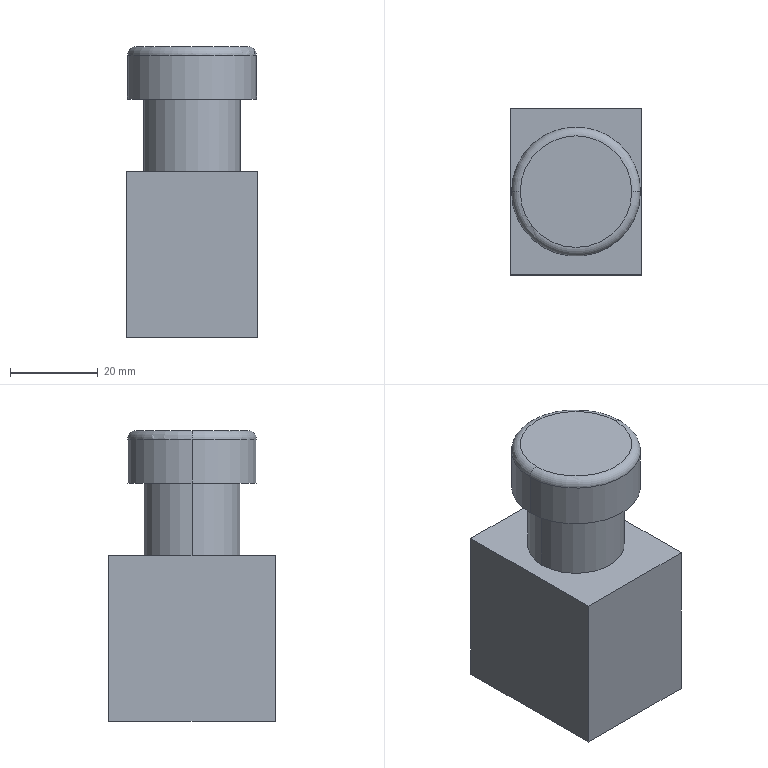Part | STEP file | illuminated flat push button white 24V | 1 solid | 14 faces | box 30 x 38 x 66.5 mm | volume 57717 mm3 | plane 8 | cylinder 4 | torus 2 | commonest cylinder face diameters 22 x2 29.5 x2
STEP:
#1=CARTESIAN_POINT('',(0.,0.,0.));
#2=DIRECTION('',(0.,0.,1.));
#3=DIRECTION('',(1.,0.,0.));
#4=AXIS2_PLACEMENT_3D('',#1,#2,#3);
#5=CARTESIAN_POINT('',(-14.75,0.,10.));
#6=VERTEX_POINT('',#5);
#7=CARTESIAN_POINT('',(14.75,0.,10.));
#8=VERTEX_POINT('',#7);
#9=CARTESIAN_POINT('',(0.,0.,10.));
#10=DIRECTION('',(0.,0.,-1.));
#11=DIRECTION('',(1.,0.,0.));
#12=AXIS2_PLACEMENT_3D('',#9,#10,#11);
#13=CIRCLE('',#12,14.75);
#14=CARTESIAN_POINT('',(0.,0.,10.));
#15=DIRECTION('',(0.,0.,1.));
#16=DIRECTION('',(1.,0.,0.));
#17=AXIS2_PLACEMENT_3D('',#14,#15,#16);
#18=TOROIDAL_SURFACE('',#17,12.75,2.);
#19=CARTESIAN_POINT('',(6.283,0.));
#20=DIRECTION('',(-1.,0.));
#21=VECTOR('',#20,1.);
#22=LINE('',#19,#21);
#23=(GEOMETRIC_REPRESENTATION_CONTEXT(2)PARAMETRIC_REPRESENTATION_CONTEXT()REPRESENTATION_CONTEXT('',''));
#24=DEFINITIONAL_REPRESENTATION('',(#22),#23);
#25=PCURVE('',#18,#24);
#26=CARTESIAN_POINT('',(0.,0.,12.));
#27=DIRECTION('',(0.,0.,-1.));
#28=DIRECTION('',(-1.,0.,0.));
#29=AXIS2_PLACEMENT_3D('',#26,#27,#28);
#30=CYLINDRICAL_SURFACE('',#29,14.75);
#31=CARTESIAN_POINT('',(-3.142,2.));
#32=DIRECTION('',(1.,0.));
#33=VECTOR('',#32,1.);
#34=LINE('',#31,#33);
#35=(GEOMETRIC_REPRESENTATION_CONTEXT(2)PARAMETRIC_REPRESENTATION_CONTEXT()REPRESENTATION_CONTEXT('',''));
#36=DEFINITIONAL_REPRESENTATION('',(#34),#35);
#37=PCURVE('',#30,#36);
#38=SURFACE_CURVE('',#13,(#25,#37),.PCURVE_S1.);
#39=EDGE_CURVE('',#6,#8,#38,.T.);
#40=ORIENTED_EDGE('',*,*,#39,.F.);
#41=CARTESIAN_POINT('',(-12.75,0.,12.));
#42=VERTEX_POINT('',#41);
#43=CARTESIAN_POINT('',(-12.75,0.,10.));
#44=DIRECTION('',(0.,1.,0.));
#45=DIRECTION('',(-1.,0.,0.));
#46=AXIS2_PLACEMENT_3D('',#43,#44,#45);
#47=CIRCLE('',#46,2.);
#48=CARTESIAN_POINT('',(3.142,0.));
#49=DIRECTION('',(0.,1.));
#50=VECTOR('',#49,1.);
#51=LINE('',#48,#50);
#52=(GEOMETRIC_REPRESENTATION_CONTEXT(2)PARAMETRIC_REPRESENTATION_CONTEXT()REPRESENTATION_CONTEXT('',''));
#53=DEFINITIONAL_REPRESENTATION('',(#51),#52);
#54=PCURVE('',#18,#53);
#55=CARTESIAN_POINT('',(0.,0.,10.));
#56=DIRECTION('',(0.,0.,1.));
#57=DIRECTION('',(1.,0.,0.));
#58=AXIS2_PLACEMENT_3D('',#55,#56,#57);
#59=TOROIDAL_SURFACE('',#58,12.75,2.);
#60=CARTESIAN_POINT('',(3.142,0.));
#61=DIRECTION('',(0.,1.));
#62=VECTOR('',#61,1.);
#63=LINE('',#60,#62);
#64=(GEOMETRIC_REPRESENTATION_CONTEXT(2)PARAMETRIC_REPRESENTATION_CONTEXT()REPRESENTATION_CONTEXT('',''));
#65=DEFINITIONAL_REPRESENTATION('',(#63),#64);
#66=PCURVE('',#59,#65);
#67=SURFACE_CURVE('',#47,(#54,#66),.PCURVE_S1.);
#68=EDGE_CURVE('',#6,#42,#67,.T.);
#69=ORIENTED_EDGE('',*,*,#68,.T.);
#70=CARTESIAN_POINT('',(12.75,0.,12.));
#71=VERTEX_POINT('',#70);
#72=CARTESIAN_POINT('',(0.,0.,12.));
#73=DIRECTION('',(0.,0.,1.));
#74=DIRECTION('',(1.,0.,0.));
#75=AXIS2_PLACEMENT_3D('',#72,#73,#74);
#76=CIRCLE('',#75,12.75);
#77=CARTESIAN_POINT('',(0.,1.571));
#78=DIRECTION('',(1.,0.));
#79=VECTOR('',#78,1.);
#80=LINE('',#77,#79);
#81=(GEOMETRIC_REPRESENTATION_CONTEXT(2)PARAMETRIC_REPRESENTATION_CONTEXT()REPRESENTATION_CONTEXT('',''));
#82=DEFINITIONAL_REPRESENTATION('',(#80),#81);
#83=PCURVE('',#18,#82);
#84=CARTESIAN_POINT('',(0.,0.,12.));
#85=DIRECTION('',(0.,0.,1.));
#86=DIRECTION('',(1.,0.,0.));
#87=AXIS2_PLACEMENT_3D('',#84,#85,#86);
#88=PLANE('',#87);
#89=CARTESIAN_POINT('',(0.,0.));
#90=DIRECTION('',(1.,0.));
#91=AXIS2_PLACEMENT_2D('',#89,#90);
#92=CIRCLE('',#91,12.75);
#93=(GEOMETRIC_REPRESENTATION_CONTEXT(2)PARAMETRIC_REPRESENTATION_CONTEXT()REPRESENTATION_CONTEXT('',''));
#94=DEFINITIONAL_REPRESENTATION('',(#92),#93);
#95=PCURVE('',#88,#94);
#96=SURFACE_CURVE('',#76,(#83,#95),.PCURVE_S1.);
#97=EDGE_CURVE('',#71,#42,#96,.T.);
#98=ORIENTED_EDGE('',*,*,#97,.F.);
#99=CARTESIAN_POINT('',(12.75,0.,10.));
#100=DIRECTION('',(0.,-1.,0.));
#101=DIRECTION('',(0.,0.,-1.));
#102=AXIS2_PLACEMENT_3D('',#99,#100,#101);
#103=CIRCLE('',#102,2.);
#104=CARTESIAN_POINT('',(0.,-1.571));
#105=DIRECTION('',(0.,1.));
#106=VECTOR('',#105,1.);
#107=LINE('',#104,#106);
#108=(GEOMETRIC_REPRESENTATION_CONTEXT(2)PARAMETRIC_REPRESENTATION_CONTEXT()REPRESENTATION_CONTEXT('',''));
#109=DEFINITIONAL_REPRESENTATION('',(#107),#108);
#110=PCURVE('',#18,#109);
#111=CARTESIAN_POINT('',(6.283,-1.571));
#112=DIRECTION('',(0.,1.));
#113=VECTOR('',#112,1.);
#114=LINE('',#111,#113);
#115=(GEOMETRIC_REPRESENTATION_CONTEXT(2)PARAMETRIC_REPRESENTATION_CONTEXT()REPRESENTATION_CONTEXT('',''));
#116=DEFINITIONAL_REPRESENTATION('',(#114),#115);
#117=PCURVE('',#59,#116);
#118=SURFACE_CURVE('',#103,(#110,#117),.PCURVE_S1.);
#119=EDGE_CURVE('',#8,#71,#118,.T.);
#120=ORIENTED_EDGE('',*,*,#119,.F.);
#121=EDGE_LOOP('',(#40,#69,#98,#120));
#122=FACE_BOUND('',#121,.T.);
#123=ADVANCED_FACE('',(#122),#18,.T.);
#124=CARTESIAN_POINT('',(-11.,0.,-16.5));
#125=VERTEX_POINT('',#124);
#126=CARTESIAN_POINT('',(11.,0.,-16.5));
#127=VERTEX_POINT('',#126);
#128=CARTESIAN_POINT('',(0.,0.,-16.5));
#129=DIRECTION('',(0.,0.,-1.));
#130=DIRECTION('',(-1.,0.,0.));
#131=AXIS2_PLACEMENT_3D('',#128,#129,#130);
#132=CIRCLE('',#131,11.);
#133=CARTESIAN_POINT('',(0.,0.,-16.5));
#134=DIRECTION('',(0.,0.,1.));
#135=DIRECTION('',(1.,0.,0.));
#136=AXIS2_PLACEMENT_3D('',#133,#134,#135);
#137=CYLINDRICAL_SURFACE('',#136,11.);
#138=CARTESIAN_POINT('',(3.142,0.));
#139=DIRECTION('',(-1.,0.));
#140=VECTOR('',#139,1.);
#141=LINE('',#138,#140);
#142=(GEOMETRIC_REPRESENTATION_CONTEXT(2)PARAMETRIC_REPRESENTATION_CONTEXT()REPRESENTATION_CONTEXT('',''));
#143=DEFINITIONAL_REPRESENTATION('',(#141),#142);
#144=PCURVE('',#137,#143);
#145=CARTESIAN_POINT('',(0.,0.,-16.5));
#146=DIRECTION('',(0.,0.,-1.));
#147=DIRECTION('',(-1.,0.,0.));
#148=AXIS2_PLACEMENT_3D('',#145,#146,#147);
#149=PLANE('',#148);
#150=CARTESIAN_POINT('',(0.,0.));
#151=DIRECTION('',(1.,0.));
#152=AXIS2_PLACEMENT_2D('',#150,#151);
#153=CIRCLE('',#152,11.);
#154=(GEOMETRIC_REPRESENTATION_CONTEXT(2)PARAMETRIC_REPRESENTATION_CONTEXT()REPRESENTATION_CONTEXT('',''));
#155=DEFINITIONAL_REPRESENTATION('',(#153),#154);
#156=PCURVE('',#149,#155);
#157=SURFACE_CURVE('',#132,(#144,#156),.PCURVE_S1.);
#158=EDGE_CURVE('',#125,#127,#157,.T.);
#159=ORIENTED_EDGE('',*,*,#158,.F.);
#160=CARTESIAN_POINT('',(-11.,0.,0.));
#161=VERTEX_POINT('',#160);
#162=CARTESIAN_POINT('',(-11.,0.,-16.5));
#163=DIRECTION('',(0.,0.,1.));
#164=VECTOR('',#163,1.);
#165=LINE('',#162,#164);
#166=CARTESIAN_POINT('',(3.142,0.));
#167=DIRECTION('',(0.,1.));
#168=VECTOR('',#167,1.);
#169=LINE('',#166,#168);
#170=(GEOMETRIC_REPRESENTATION_CONTEXT(2)PARAMETRIC_REPRESENTATION_CONTEXT()REPRESENTATION_CONTEXT('',''));
#171=DEFINITIONAL_REPRESENTATION('',(#169),#170);
#172=PCURVE('',#137,#171);
#173=CARTESIAN_POINT('',(0.,0.,-16.5));
#174=DIRECTION('',(0.,0.,1.));
#175=DIRECTION('',(1.,0.,0.));
#176=AXIS2_PLACEMENT_3D('',#173,#174,#175);
#177=CYLINDRICAL_SURFACE('',#176,11.);
#178=CARTESIAN_POINT('',(3.142,0.));
#179=DIRECTION('',(0.,1.));
#180=VECTOR('',#179,1.);
#181=LINE('',#178,#180);
#182=(GEOMETRIC_REPRESENTATION_CONTEXT(2)PARAMETRIC_REPRESENTATION_CONTEXT()REPRESENTATION_CONTEXT('',''));
#183=DEFINITIONAL_REPRESENTATION('',(#181),#182);
#184=PCURVE('',#177,#183);
#185=SURFACE_CURVE('',#165,(#172,#184),.PCURVE_S1.);
#186=EDGE_CURVE('',#125,#161,#185,.T.);
#187=ORIENTED_EDGE('',*,*,#186,.T.);
#188=CARTESIAN_POINT('',(11.,0.,0.));
#189=VERTEX_POINT('',#188);
#190=CARTESIAN_POINT('',(0.,0.,0.));
#191=DIRECTION('',(0.,0.,-1.));
#192=DIRECTION('',(-1.,0.,0.));
#193=AXIS2_PLACEMENT_3D('',#190,#191,#192);
#194=CIRCLE('',#193,11.);
#195=CARTESIAN_POINT('',(3.142,16.5));
#196=DIRECTION('',(-1.,0.));
#197=VECTOR('',#196,1.);
#198=LINE('',#195,#197);
#199=(GEOMETRIC_REPRESENTATION_CONTEXT(2)PARAMETRIC_REPRESENTATION_CONTEXT()REPRESENTATION_CONTEXT('',''));
#200=DEFINITIONAL_REPRESENTATION('',(#198),#199);
#201=PCURVE('',#137,#200);
#202=CARTESIAN_POINT('',(0.,0.,0.));
#203=DIRECTION('',(0.,0.,1.));
#204=DIRECTION('',(1.,0.,0.));
#205=AXIS2_PLACEMENT_3D('',#202,#203,#204);
#206=PLANE('',#205);
#207=CARTESIAN_POINT('',(-11.,0.));
#208=CARTESIAN_POINT('',(-11.,19.053));
#209=CARTESIAN_POINT('',(5.5,9.526));
#210=CARTESIAN_POINT('',(22.,0.));
#211=CARTESIAN_POINT('',(5.5,-9.526));
#212=CARTESIAN_POINT('',(-11.,-19.053));
#213=CARTESIAN_POINT('',(-11.,0.));
#214=(BOUNDED_CURVE()B_SPLINE_CURVE(2,(#207,#208,#209,#210,#211,#212,#213),.UNSPECIFIED.,.T.,.F.)B_SPLINE_CURVE_WITH_KNOTS((1,2,2,2,2,1),(-2.094,0.,2.094,4.189,6.283,8.378),.UNSPECIFIED.)CURVE()GEOMETRIC_REPRESENTATION_ITEM()RATIONAL_B_SPLINE_CURVE((1.,0.5,1.,0.5,1.,0.5,1.))REPRESENTATION_ITEM(''));
#215=(GEOMETRIC_REPRESENTATION_CONTEXT(2)PARAMETRIC_REPRESENTATION_CONTEXT()REPRESENTATION_CONTEXT('',''));
#216=DEFINITIONAL_REPRESENTATION('',(#214),#215);
#217=PCURVE('',#206,#216);
#218=SURFACE_CURVE('',#194,(#201,#217),.PCURVE_S1.);
#219=EDGE_CURVE('',#161,#189,#218,.T.);
#220=ORIENTED_EDGE('',*,*,#219,.T.);
#221=CARTESIAN_POINT('',(11.,0.,-16.5));
#222=DIRECTION('',(0.,0.,1.));
#223=VECTOR('',#222,1.);
#224=LINE('',#221,#223);
#225=CARTESIAN_POINT('',(0.,0.));
#226=DIRECTION('',(0.,1.));
#227=VECTOR('',#226,1.);
#228=LINE('',#225,#227);
#229=(GEOMETRIC_REPRESENTATION_CONTEXT(2)PARAMETRIC_REPRESENTATION_CONTEXT()REPRESENTATION_CONTEXT('',''));
#230=DEFINITIONAL_REPRESENTATION('',(#228),#229);
#231=PCURVE('',#137,#230);
#232=CARTESIAN_POINT('',(6.283,0.));
#233=DIRECTION('',(0.,1.));
#234=VECTOR('',#233,1.);
#235=LINE('',#232,#234);
#236=(GEOMETRIC_REPRESENTATION_CONTEXT(2)PARAMETRIC_REPRESENTATION_CONTEXT()REPRESENTATION_CONTEXT('',''));
#237=DEFINITIONAL_REPRESENTATION('',(#235),#236);
#238=PCURVE('',#177,#237);
#239=SURFACE_CURVE('',#224,(#231,#238),.PCURVE_S1.);
#240=EDGE_CURVE('',#127,#189,#239,.T.);
#241=ORIENTED_EDGE('',*,*,#240,.F.);
#242=EDGE_LOOP('',(#159,#187,#220,#241));
#243=FACE_BOUND('',#242,.T.);
#244=ADVANCED_FACE('',(#243),#137,.T.);
#245=ORIENTED_EDGE('',*,*,#39,.T.);
#246=CARTESIAN_POINT('',(14.75,0.,0.));
#247=VERTEX_POINT('',#246);
#248=CARTESIAN_POINT('',(14.75,0.,12.));
#249=DIRECTION('',(0.,0.,-1.));
#250=VECTOR('',#249,1.);
#251=LINE('',#248,#250);
#252=CARTESIAN_POINT('',(3.142,0.));
#253=DIRECTION('',(0.,1.));
#254=VECTOR('',#253,1.);
#255=LINE('',#252,#254);
#256=(GEOMETRIC_REPRESENTATION_CONTEXT(2)PARAMETRIC_REPRESENTATION_CONTEXT()REPRESENTATION_CONTEXT('',''));
#257=DEFINITIONAL_REPRESENTATION('',(#255),#256);
#258=PCURVE('',#30,#257);
#259=CARTESIAN_POINT('',(0.,0.,12.));
#260=DIRECTION('',(0.,0.,-1.));
#261=DIRECTION('',(-1.,0.,0.));
#262=AXIS2_PLACEMENT_3D('',#259,#260,#261);
#263=CYLINDRICAL_SURFACE('',#262,14.75);
#264=CARTESIAN_POINT('',(3.142,0.));
#265=DIRECTION('',(0.,1.));
#266=VECTOR('',#265,1.);
#267=LINE('',#264,#266);
#268=(GEOMETRIC_REPRESENTATION_CONTEXT(2)PARAMETRIC_REPRESENTATION_CONTEXT()REPRESENTATION_CONTEXT('',''));
#269=DEFINITIONAL_REPRESENTATION('',(#267),#268);
#270=PCURVE('',#263,#269);
#271=SURFACE_CURVE('',#251,(#258,#270),.PCURVE_S1.);
#272=EDGE_CURVE('',#8,#247,#271,.T.);
#273=ORIENTED_EDGE('',*,*,#272,.T.);
#274=CARTESIAN_POINT('',(-14.75,0.,0.));
#275=VERTEX_POINT('',#274);
#276=CARTESIAN_POINT('',(0.,0.,0.));
#277=DIRECTION('',(0.,0.,1.));
#278=DIRECTION('',(1.,0.,0.));
#279=AXIS2_PLACEMENT_3D('',#276,#277,#278);
#280=CIRCLE('',#279,14.75);
#281=CARTESIAN_POINT('',(3.142,12.));
#282=DIRECTION('',(-1.,0.));
#283=VECTOR('',#282,1.);
#284=LINE('',#281,#283);
#285=(GEOMETRIC_REPRESENTATION_CONTEXT(2)PARAMETRIC_REPRESENTATION_CONTEXT()REPRESENTATION_CONTEXT('',''));
#286=DEFINITIONAL_REPRESENTATION('',(#284),#285);
#287=PCURVE('',#30,#286);
#288=CARTESIAN_POINT('',(0.,0.));
#289=DIRECTION('',(1.,0.));
#290=AXIS2_PLACEMENT_2D('',#288,#289);
#291=CIRCLE('',#290,14.75);
#292=(GEOMETRIC_REPRESENTATION_CONTEXT(2)PARAMETRIC_REPRESENTATION_CONTEXT()REPRESENTATION_CONTEXT('',''));
#293=DEFINITIONAL_REPRESENTATION('',(#291),#292);
#294=PCURVE('',#206,#293);
#295=SURFACE_CURVE('',#280,(#287,#294),.PCURVE_S1.);
#296=EDGE_CURVE('',#247,#275,#295,.T.);
#297=ORIENTED_EDGE('',*,*,#296,.T.);
#298=CARTESIAN_POINT('',(-14.75,0.,12.));
#299=DIRECTION('',(0.,0.,-1.));
#300=VECTOR('',#299,1.);
#301=LINE('',#298,#300);
#302=CARTESIAN_POINT('',(0.,0.));
#303=DIRECTION('',(0.,1.));
#304=VECTOR('',#303,1.);
#305=LINE('',#302,#304);
#306=(GEOMETRIC_REPRESENTATION_CONTEXT(2)PARAMETRIC_REPRESENTATION_CONTEXT()REPRESENTATION_CONTEXT('',''));
#307=DEFINITIONAL_REPRESENTATION('',(#305),#306);
#308=PCURVE('',#30,#307);
#309=CARTESIAN_POINT('',(6.283,0.));
#310=DIRECTION('',(0.,1.));
#311=VECTOR('',#310,1.);
#312=LINE('',#309,#311);
#313=(GEOMETRIC_REPRESENTATION_CONTEXT(2)PARAMETRIC_REPRESENTATION_CONTEXT()REPRESENTATION_CONTEXT('',''));
#314=DEFINITIONAL_REPRESENTATION('',(#312),#313);
#315=PCURVE('',#263,#314);
#316=SURFACE_CURVE('',#301,(#308,#315),.PCURVE_S1.);
#317=EDGE_CURVE('',#6,#275,#316,.T.);
#318=ORIENTED_EDGE('',*,*,#317,.F.);
#319=EDGE_LOOP('',(#245,#273,#297,#318));
#320=FACE_BOUND('',#319,.T.);
#321=ADVANCED_FACE('',(#320),#30,.T.);
#322=ORIENTED_EDGE('',*,*,#272,.F.);
#323=CARTESIAN_POINT('',(0.,0.,10.));
#324=DIRECTION('',(0.,0.,-1.));
#325=DIRECTION('',(1.,0.,0.));
#326=AXIS2_PLACEMENT_3D('',#323,#324,#325);
#327=CIRCLE('',#326,14.75);
#328=CARTESIAN_POINT('',(3.142,2.));
#329=DIRECTION('',(1.,0.));
#330=VECTOR('',#329,1.);
#331=LINE('',#328,#330);
#332=(GEOMETRIC_REPRESENTATION_CONTEXT(2)PARAMETRIC_REPRESENTATION_CONTEXT()REPRESENTATION_CONTEXT('',''));
#333=DEFINITIONAL_REPRESENTATION('',(#331),#332);
#334=PCURVE('',#263,#333);
#335=CARTESIAN_POINT('',(6.283,0.));
#336=DIRECTION('',(-1.,0.));
#337=VECTOR('',#336,1.);
#338=LINE('',#335,#337);
#339=(GEOMETRIC_REPRESENTATION_CONTEXT(2)PARAMETRIC_REPRESENTATION_CONTEXT()REPRESENTATION_CONTEXT('',''));
#340=DEFINITIONAL_REPRESENTATION('',(#338),#339);
#341=PCURVE('',#59,#340);
#342=SURFACE_CURVE('',#327,(#334,#341),.PCURVE_S1.);
#343=EDGE_CURVE('',#8,#6,#342,.T.);
#344=ORIENTED_EDGE('',*,*,#343,.T.);
#345=ORIENTED_EDGE('',*,*,#317,.T.);
#346=CARTESIAN_POINT('',(0.,0.,0.));
#347=DIRECTION('',(0.,0.,1.));
#348=DIRECTION('',(1.,0.,0.));
#349=AXIS2_PLACEMENT_3D('',#346,#347,#348);
#350=CIRCLE('',#349,14.75);
#351=CARTESIAN_POINT('',(9.425,12.));
#352=DIRECTION('',(-1.,0.));
#353=VECTOR('',#352,1.);
#354=LINE('',#351,#353);
#355=(GEOMETRIC_REPRESENTATION_CONTEXT(2)PARAMETRIC_REPRESENTATION_CONTEXT()REPRESENTATION_CONTEXT('',''));
#356=DEFINITIONAL_REPRESENTATION('',(#354),#355);
#357=PCURVE('',#263,#356);
#358=CARTESIAN_POINT('',(0.,0.));
#359=DIRECTION('',(1.,0.));
#360=AXIS2_PLACEMENT_2D('',#358,#359);
#361=CIRCLE('',#360,14.75);
#362=(GEOMETRIC_REPRESENTATION_CONTEXT(2)PARAMETRIC_REPRESENTATION_CONTEXT()REPRESENTATION_CONTEXT('',''));
#363=DEFINITIONAL_REPRESENTATION('',(#361),#362);
#364=PCURVE('',#206,#363);
#365=SURFACE_CURVE('',#350,(#357,#364),.PCURVE_S1.);
#366=EDGE_CURVE('',#275,#247,#365,.T.);
#367=ORIENTED_EDGE('',*,*,#366,.T.);
#368=EDGE_LOOP('',(#322,#344,#345,#367));
#369=FACE_BOUND('',#368,.T.);
#370=ADVANCED_FACE('',(#369),#263,.T.);
#371=ORIENTED_EDGE('',*,*,#97,.T.);
#372=CARTESIAN_POINT('',(0.,0.,12.));
#373=DIRECTION('',(0.,0.,1.));
#374=DIRECTION('',(1.,0.,0.));
#375=AXIS2_PLACEMENT_3D('',#372,#373,#374);
#376=CIRCLE('',#375,12.75);
#377=CARTESIAN_POINT('',(0.,0.));
#378=DIRECTION('',(1.,0.));
#379=AXIS2_PLACEMENT_2D('',#377,#378);
#380=CIRCLE('',#379,12.75);
#381=(GEOMETRIC_REPRESENTATION_CONTEXT(2)PARAMETRIC_REPRESENTATION_CONTEXT()REPRESENTATION_CONTEXT('',''));
#382=DEFINITIONAL_REPRESENTATION('',(#380),#381);
#383=PCURVE('',#88,#382);
#384=CARTESIAN_POINT('',(0.,1.571));
#385=DIRECTION('',(1.,0.));
#386=VECTOR('',#385,1.);
#387=LINE('',#384,#386);
#388=(GEOMETRIC_REPRESENTATION_CONTEXT(2)PARAMETRIC_REPRESENTATION_CONTEXT()REPRESENTATION_CONTEXT('',''));
#389=DEFINITIONAL_REPRESENTATION('',(#387),#388);
#390=PCURVE('',#59,#389);
#391=SURFACE_CURVE('',#376,(#383,#390),.PCURVE_S1.);
#392=EDGE_CURVE('',#42,#71,#391,.T.);
#393=ORIENTED_EDGE('',*,*,#392,.T.);
#394=EDGE_LOOP('',(#371,#393));
#395=FACE_BOUND('',#394,.T.);
#396=ADVANCED_FACE('',(#395),#88,.T.);
#397=CARTESIAN_POINT('',(0.,0.,0.));
#398=DIRECTION('',(0.,0.,-1.));
#399=DIRECTION('',(-1.,0.,0.));
#400=AXIS2_PLACEMENT_3D('',#397,#398,#399);
#401=CIRCLE('',#400,11.);
#402=CARTESIAN_POINT('',(-11.,0.));
#403=CARTESIAN_POINT('',(-11.,19.053));
#404=CARTESIAN_POINT('',(5.5,9.526));
#405=CARTESIAN_POINT('',(22.,0.));
#406=CARTESIAN_POINT('',(5.5,-9.526));
#407=CARTESIAN_POINT('',(-11.,-19.053));
#408=CARTESIAN_POINT('',(-11.,0.));
#409=(BOUNDED_CURVE()B_SPLINE_CURVE(2,(#402,#403,#404,#405,#406,#407,#408),.UNSPECIFIED.,.T.,.F.)B_SPLINE_CURVE_WITH_KNOTS((1,2,2,2,2,1),(-2.094,0.,2.094,4.189,6.283,8.378),.UNSPECIFIED.)CURVE()GEOMETRIC_REPRESENTATION_ITEM()RATIONAL_B_SPLINE_CURVE((1.,0.5,1.,0.5,1.,0.5,1.))REPRESENTATION_ITEM(''));
#410=(GEOMETRIC_REPRESENTATION_CONTEXT(2)PARAMETRIC_REPRESENTATION_CONTEXT()REPRESENTATION_CONTEXT('',''));
#411=DEFINITIONAL_REPRESENTATION('',(#409),#410);
#412=PCURVE('',#206,#411);
#413=CARTESIAN_POINT('',(9.425,16.5));
#414=DIRECTION('',(-1.,0.));
#415=VECTOR('',#414,1.);
#416=LINE('',#413,#415);
#417=(GEOMETRIC_REPRESENTATION_CONTEXT(2)PARAMETRIC_REPRESENTATION_CONTEXT()REPRESENTATION_CONTEXT('',''));
#418=DEFINITIONAL_REPRESENTATION('',(#416),#417);
#419=PCURVE('',#177,#418);
#420=SURFACE_CURVE('',#401,(#412,#419),.PCURVE_S1.);
#421=EDGE_CURVE('',#189,#161,#420,.T.);
#422=ORIENTED_EDGE('',*,*,#421,.F.);
#423=ORIENTED_EDGE('',*,*,#219,.F.);
#424=EDGE_LOOP('',(#422,#423));
#425=FACE_BOUND('',#424,.T.);
#426=ORIENTED_EDGE('',*,*,#366,.F.);
#427=ORIENTED_EDGE('',*,*,#296,.F.);
#428=EDGE_LOOP('',(#426,#427));
#429=FACE_BOUND('',#428,.T.);
#430=ADVANCED_FACE('',(#425,#429),#206,.F.);
#431=ORIENTED_EDGE('',*,*,#186,.F.);
#432=CARTESIAN_POINT('',(0.,0.,-16.5));
#433=DIRECTION('',(0.,0.,-1.));
#434=DIRECTION('',(-1.,0.,0.));
#435=AXIS2_PLACEMENT_3D('',#432,#433,#434);
#436=CIRCLE('',#435,11.);
#437=CARTESIAN_POINT('',(9.425,0.));
#438=DIRECTION('',(-1.,0.));
#439=VECTOR('',#438,1.);
#440=LINE('',#437,#439);
#441=(GEOMETRIC_REPRESENTATION_CONTEXT(2)PARAMETRIC_REPRESENTATION_CONTEXT()REPRESENTATION_CONTEXT('',''));
#442=DEFINITIONAL_REPRESENTATION('',(#440),#441);
#443=PCURVE('',#177,#442);
#444=CARTESIAN_POINT('',(0.,0.));
#445=DIRECTION('',(1.,0.));
#446=AXIS2_PLACEMENT_2D('',#444,#445);
#447=CIRCLE('',#446,11.);
#448=(GEOMETRIC_REPRESENTATION_CONTEXT(2)PARAMETRIC_REPRESENTATION_CONTEXT()REPRESENTATION_CONTEXT('',''));
#449=DEFINITIONAL_REPRESENTATION('',(#447),#448);
#450=PCURVE('',#149,#449);
#451=SURFACE_CURVE('',#436,(#443,#450),.PCURVE_S1.);
#452=EDGE_CURVE('',#127,#125,#451,.T.);
#453=ORIENTED_EDGE('',*,*,#452,.F.);
#454=ORIENTED_EDGE('',*,*,#240,.T.);
#455=ORIENTED_EDGE('',*,*,#421,.T.);
#456=EDGE_LOOP('',(#431,#453,#454,#455));
#457=FACE_BOUND('',#456,.T.);
#458=ADVANCED_FACE('',(#457),#177,.T.);
#459=ORIENTED_EDGE('',*,*,#68,.F.);
#460=ORIENTED_EDGE('',*,*,#343,.F.);
#461=ORIENTED_EDGE('',*,*,#119,.T.);
#462=ORIENTED_EDGE('',*,*,#392,.F.);
#463=EDGE_LOOP('',(#459,#460,#461,#462));
#464=FACE_BOUND('',#463,.T.);
#465=ADVANCED_FACE('',(#464),#59,.T.);
#466=CARTESIAN_POINT('',(15.,19.,-16.5));
#467=VERTEX_POINT('',#466);
#468=CARTESIAN_POINT('',(15.,-19.,-16.5));
#469=VERTEX_POINT('',#468);
#470=CARTESIAN_POINT('',(15.,19.,-16.5));
#471=DIRECTION('',(0.,-1.,0.));
#472=VECTOR('',#471,1.);
#473=LINE('',#470,#472);
#474=CARTESIAN_POINT('',(15.,19.,-54.5));
#475=DIRECTION('',(-1.,0.,0.));
#476=DIRECTION('',(0.,0.,1.));
#477=AXIS2_PLACEMENT_3D('',#474,#475,#476);
#478=PLANE('',#477);
#479=CARTESIAN_POINT('',(38.,0.));
#480=DIRECTION('',(0.,-1.));
#481=VECTOR('',#480,1.);
#482=LINE('',#479,#481);
#483=(GEOMETRIC_REPRESENTATION_CONTEXT(2)PARAMETRIC_REPRESENTATION_CONTEXT()REPRESENTATION_CONTEXT('',''));
#484=DEFINITIONAL_REPRESENTATION('',(#482),#483);
#485=PCURVE('',#478,#484);
#486=CARTESIAN_POINT('',(-15.,19.));
#487=DIRECTION('',(0.,-1.));
#488=VECTOR('',#487,1.);
#489=LINE('',#486,#488);
#490=(GEOMETRIC_REPRESENTATION_CONTEXT(2)PARAMETRIC_REPRESENTATION_CONTEXT()REPRESENTATION_CONTEXT('',''));
#491=DEFINITIONAL_REPRESENTATION('',(#489),#490);
#492=PCURVE('',#149,#491);
#493=SURFACE_CURVE('',#473,(#485,#492),.PCURVE_S1.);
#494=EDGE_CURVE('',#467,#469,#493,.T.);
#495=ORIENTED_EDGE('',*,*,#494,.T.);
#496=CARTESIAN_POINT('',(15.,-19.,-54.5));
#497=VERTEX_POINT('',#496);
#498=CARTESIAN_POINT('',(15.,-19.,-54.5));
#499=DIRECTION('',(0.,0.,1.));
#500=VECTOR('',#499,1.);
#501=LINE('',#498,#500);
#502=CARTESIAN_POINT('',(0.,-38.));
#503=DIRECTION('',(1.,0.));
#504=VECTOR('',#503,1.);
#505=LINE('',#502,#504);
#506=(GEOMETRIC_REPRESENTATION_CONTEXT(2)PARAMETRIC_REPRESENTATION_CONTEXT()REPRESENTATION_CONTEXT('',''));
#507=DEFINITIONAL_REPRESENTATION('',(#505),#506);
#508=PCURVE('',#478,#507);
#509=CARTESIAN_POINT('',(15.,-19.,-54.5));
#510=DIRECTION('',(0.,1.,0.));
#511=DIRECTION('',(-1.,0.,0.));
#512=AXIS2_PLACEMENT_3D('',#509,#510,#511);
#513=PLANE('',#512);
#514=CARTESIAN_POINT('',(0.,0.));
#515=DIRECTION('',(0.,1.));
#516=VECTOR('',#515,1.);
#517=LINE('',#514,#516);
#518=(GEOMETRIC_REPRESENTATION_CONTEXT(2)PARAMETRIC_REPRESENTATION_CONTEXT()REPRESENTATION_CONTEXT('',''));
#519=DEFINITIONAL_REPRESENTATION('',(#517),#518);
#520=PCURVE('',#513,#519);
#521=SURFACE_CURVE('',#501,(#508,#520),.PCURVE_S1.);
#522=EDGE_CURVE('',#497,#469,#521,.T.);
#523=ORIENTED_EDGE('',*,*,#522,.F.);
#524=CARTESIAN_POINT('',(15.,19.,-54.5));
#525=VERTEX_POINT('',#524);
#526=CARTESIAN_POINT('',(15.,19.,-54.5));
#527=DIRECTION('',(0.,-1.,0.));
#528=VECTOR('',#527,1.);
#529=LINE('',#526,#528);
#530=CARTESIAN_POINT('',(0.,0.));
#531=DIRECTION('',(0.,-1.));
#532=VECTOR('',#531,1.);
#533=LINE('',#530,#532);
#534=(GEOMETRIC_REPRESENTATION_CONTEXT(2)PARAMETRIC_REPRESENTATION_CONTEXT()REPRESENTATION_CONTEXT('',''));
#535=DEFINITIONAL_REPRESENTATION('',(#533),#534);
#536=PCURVE('',#478,#535);
#537=CARTESIAN_POINT('',(0.,0.,-54.5));
#538=DIRECTION('',(0.,0.,-1.));
#539=DIRECTION('',(-1.,0.,0.));
#540=AXIS2_PLACEMENT_3D('',#537,#538,#539);
#541=PLANE('',#540);
#542=CARTESIAN_POINT('',(-15.,19.));
#543=DIRECTION('',(0.,-1.));
#544=VECTOR('',#543,1.);
#545=LINE('',#542,#544);
#546=(GEOMETRIC_REPRESENTATION_CONTEXT(2)PARAMETRIC_REPRESENTATION_CONTEXT()REPRESENTATION_CONTEXT('',''));
#547=DEFINITIONAL_REPRESENTATION('',(#545),#546);
#548=PCURVE('',#541,#547);
#549=SURFACE_CURVE('',#529,(#536,#548),.PCURVE_S1.);
#550=EDGE_CURVE('',#525,#497,#549,.T.);
#551=ORIENTED_EDGE('',*,*,#550,.F.);
#552=CARTESIAN_POINT('',(15.,19.,-54.5));
#553=DIRECTION('',(0.,0.,1.));
#554=VECTOR('',#553,1.);
#555=LINE('',#552,#554);
#556=CARTESIAN_POINT('',(0.,0.));
#557=DIRECTION('',(1.,0.));
#558=VECTOR('',#557,1.);
#559=LINE('',#556,#558);
#560=(GEOMETRIC_REPRESENTATION_CONTEXT(2)PARAMETRIC_REPRESENTATION_CONTEXT()REPRESENTATION_CONTEXT('',''));
#561=DEFINITIONAL_REPRESENTATION('',(#559),#560);
#562=PCURVE('',#478,#561);
#563=CARTESIAN_POINT('',(15.,19.,-54.5));
#564=DIRECTION('',(0.,-1.,0.));
#565=DIRECTION('',(1.,0.,0.));
#566=AXIS2_PLACEMENT_3D('',#563,#564,#565);
#567=PLANE('',#566);
#568=CARTESIAN_POINT('',(0.,0.));
#569=DIRECTION('',(0.,1.));
#570=VECTOR('',#569,1.);
#571=LINE('',#568,#570);
#572=(GEOMETRIC_REPRESENTATION_CONTEXT(2)PARAMETRIC_REPRESENTATION_CONTEXT()REPRESENTATION_CONTEXT('',''));
#573=DEFINITIONAL_REPRESENTATION('',(#571),#572);
#574=PCURVE('',#567,#573);
#575=SURFACE_CURVE('',#555,(#562,#574),.PCURVE_S1.);
#576=EDGE_CURVE('',#525,#467,#575,.T.);
#577=ORIENTED_EDGE('',*,*,#576,.T.);
#578=EDGE_LOOP('',(#495,#523,#551,#577));
#579=FACE_BOUND('',#578,.T.);
#580=ADVANCED_FACE('',(#579),#478,.F.);
#581=CARTESIAN_POINT('',(-15.,-19.,-16.5));
#582=VERTEX_POINT('',#581);
#583=CARTESIAN_POINT('',(15.,-19.,-16.5));
#584=DIRECTION('',(-1.,0.,0.));
#585=VECTOR('',#584,1.);
#586=LINE('',#583,#585);
#587=CARTESIAN_POINT('',(0.,38.));
#588=DIRECTION('',(1.,0.));
#589=VECTOR('',#588,1.);
#590=LINE('',#587,#589);
#591=(GEOMETRIC_REPRESENTATION_CONTEXT(2)PARAMETRIC_REPRESENTATION_CONTEXT()REPRESENTATION_CONTEXT('',''));
#592=DEFINITIONAL_REPRESENTATION('',(#590),#591);
#593=PCURVE('',#513,#592);
#594=CARTESIAN_POINT('',(-15.,-19.));
#595=DIRECTION('',(1.,0.));
#596=VECTOR('',#595,1.);
#597=LINE('',#594,#596);
#598=(GEOMETRIC_REPRESENTATION_CONTEXT(2)PARAMETRIC_REPRESENTATION_CONTEXT()REPRESENTATION_CONTEXT('',''));
#599=DEFINITIONAL_REPRESENTATION('',(#597),#598);
#600=PCURVE('',#149,#599);
#601=SURFACE_CURVE('',#586,(#593,#600),.PCURVE_S1.);
#602=EDGE_CURVE('',#469,#582,#601,.T.);
#603=ORIENTED_EDGE('',*,*,#602,.T.);
#604=CARTESIAN_POINT('',(-15.,-19.,-54.5));
#605=VERTEX_POINT('',#604);
#606=CARTESIAN_POINT('',(-15.,-19.,-54.5));
#607=DIRECTION('',(0.,0.,1.));
#608=VECTOR('',#607,1.);
#609=LINE('',#606,#608);
#610=CARTESIAN_POINT('',(30.,0.));
#611=DIRECTION('',(0.,1.));
#612=VECTOR('',#611,1.);
#613=LINE('',#610,#612);
#614=(GEOMETRIC_REPRESENTATION_CONTEXT(2)PARAMETRIC_REPRESENTATION_CONTEXT()REPRESENTATION_CONTEXT('',''));
#615=DEFINITIONAL_REPRESENTATION('',(#613),#614);
#616=PCURVE('',#513,#615);
#617=CARTESIAN_POINT('',(-15.,19.,-54.5));
#618=DIRECTION('',(1.,0.,0.));
#619=DIRECTION('',(0.,1.,0.));
#620=AXIS2_PLACEMENT_3D('',#617,#618,#619);
#621=PLANE('',#620);
#622=CARTESIAN_POINT('',(-38.,0.));
#623=DIRECTION('',(0.,1.));
#624=VECTOR('',#623,1.);
#625=LINE('',#622,#624);
#626=(GEOMETRIC_REPRESENTATION_CONTEXT(2)PARAMETRIC_REPRESENTATION_CONTEXT()REPRESENTATION_CONTEXT('',''));
#627=DEFINITIONAL_REPRESENTATION('',(#625),#626);
#628=PCURVE('',#621,#627);
#629=SURFACE_CURVE('',#609,(#616,#628),.PCURVE_S1.);
#630=EDGE_CURVE('',#605,#582,#629,.T.);
#631=ORIENTED_EDGE('',*,*,#630,.F.);
#632=CARTESIAN_POINT('',(15.,-19.,-54.5));
#633=DIRECTION('',(-1.,0.,0.));
#634=VECTOR('',#633,1.);
#635=LINE('',#632,#634);
#636=CARTESIAN_POINT('',(0.,0.));
#637=DIRECTION('',(1.,0.));
#638=VECTOR('',#637,1.);
#639=LINE('',#636,#638);
#640=(GEOMETRIC_REPRESENTATION_CONTEXT(2)PARAMETRIC_REPRESENTATION_CONTEXT()REPRESENTATION_CONTEXT('',''));
#641=DEFINITIONAL_REPRESENTATION('',(#639),#640);
#642=PCURVE('',#513,#641);
#643=CARTESIAN_POINT('',(-15.,-19.));
#644=DIRECTION('',(1.,0.));
#645=VECTOR('',#644,1.);
#646=LINE('',#643,#645);
#647=(GEOMETRIC_REPRESENTATION_CONTEXT(2)PARAMETRIC_REPRESENTATION_CONTEXT()REPRESENTATION_CONTEXT('',''));
#648=DEFINITIONAL_REPRESENTATION('',(#646),#647);
#649=PCURVE('',#541,#648);
#650=SURFACE_CURVE('',#635,(#642,#649),.PCURVE_S1.);
#651=EDGE_CURVE('',#497,#605,#650,.T.);
#652=ORIENTED_EDGE('',*,*,#651,.F.);
#653=ORIENTED_EDGE('',*,*,#522,.T.);
#654=EDGE_LOOP('',(#603,#631,#652,#653));
#655=FACE_BOUND('',#654,.T.);
#656=ADVANCED_FACE('',(#655),#513,.F.);
#657=CARTESIAN_POINT('',(-15.,19.,-16.5));
#658=VERTEX_POINT('',#657);
#659=CARTESIAN_POINT('',(-15.,19.,-16.5));
#660=DIRECTION('',(0.,1.,0.));
#661=VECTOR('',#660,1.);
#662=LINE('',#659,#661);
#663=CARTESIAN_POINT('',(0.,38.));
#664=DIRECTION('',(1.,0.));
#665=VECTOR('',#664,1.);
#666=LINE('',#663,#665);
#667=(GEOMETRIC_REPRESENTATION_CONTEXT(2)PARAMETRIC_REPRESENTATION_CONTEXT()REPRESENTATION_CONTEXT('',''));
#668=DEFINITIONAL_REPRESENTATION('',(#666),#667);
#669=PCURVE('',#621,#668);
#670=CARTESIAN_POINT('',(15.,19.));
#671=DIRECTION('',(0.,1.));
#672=VECTOR('',#671,1.);
#673=LINE('',#670,#672);
#674=(GEOMETRIC_REPRESENTATION_CONTEXT(2)PARAMETRIC_REPRESENTATION_CONTEXT()REPRESENTATION_CONTEXT('',''));
#675=DEFINITIONAL_REPRESENTATION('',(#673),#674);
#676=PCURVE('',#149,#675);
#677=SURFACE_CURVE('',#662,(#669,#676),.PCURVE_S1.);
#678=EDGE_CURVE('',#582,#658,#677,.T.);
#679=ORIENTED_EDGE('',*,*,#678,.T.);
#680=CARTESIAN_POINT('',(-15.,19.,-54.5));
#681=VERTEX_POINT('',#680);
#682=CARTESIAN_POINT('',(-15.,19.,-54.5));
#683=DIRECTION('',(0.,0.,1.));
#684=VECTOR('',#683,1.);
#685=LINE('',#682,#684);
#686=CARTESIAN_POINT('',(0.,0.));
#687=DIRECTION('',(0.,1.));
#688=VECTOR('',#687,1.);
#689=LINE('',#686,#688);
#690=(GEOMETRIC_REPRESENTATION_CONTEXT(2)PARAMETRIC_REPRESENTATION_CONTEXT()REPRESENTATION_CONTEXT('',''));
#691=DEFINITIONAL_REPRESENTATION('',(#689),#690);
#692=PCURVE('',#621,#691);
#693=CARTESIAN_POINT('',(-30.,0.));
#694=DIRECTION('',(0.,1.));
#695=VECTOR('',#694,1.);
#696=LINE('',#693,#695);
#697=(GEOMETRIC_REPRESENTATION_CONTEXT(2)PARAMETRIC_REPRESENTATION_CONTEXT()REPRESENTATION_CONTEXT('',''));
#698=DEFINITIONAL_REPRESENTATION('',(#696),#697);
#699=PCURVE('',#567,#698);
#700=SURFACE_CURVE('',#685,(#692,#699),.PCURVE_S1.);
#701=EDGE_CURVE('',#681,#658,#700,.T.);
#702=ORIENTED_EDGE('',*,*,#701,.F.);
#703=CARTESIAN_POINT('',(-15.,19.,-54.5));
#704=DIRECTION('',(0.,1.,0.));
#705=VECTOR('',#704,1.);
#706=LINE('',#703,#705);
#707=CARTESIAN_POINT('',(0.,0.));
#708=DIRECTION('',(1.,0.));
#709=VECTOR('',#708,1.);
#710=LINE('',#707,#709);
#711=(GEOMETRIC_REPRESENTATION_CONTEXT(2)PARAMETRIC_REPRESENTATION_CONTEXT()REPRESENTATION_CONTEXT('',''));
#712=DEFINITIONAL_REPRESENTATION('',(#710),#711);
#713=PCURVE('',#621,#712);
#714=CARTESIAN_POINT('',(15.,19.));
#715=DIRECTION('',(0.,1.));
#716=VECTOR('',#715,1.);
#717=LINE('',#714,#716);
#718=(GEOMETRIC_REPRESENTATION_CONTEXT(2)PARAMETRIC_REPRESENTATION_CONTEXT()REPRESENTATION_CONTEXT('',''));
#719=DEFINITIONAL_REPRESENTATION('',(#717),#718);
#720=PCURVE('',#541,#719);
#721=SURFACE_CURVE('',#706,(#713,#720),.PCURVE_S1.);
#722=EDGE_CURVE('',#605,#681,#721,.T.);
#723=ORIENTED_EDGE('',*,*,#722,.F.);
#724=ORIENTED_EDGE('',*,*,#630,.T.);
#725=EDGE_LOOP('',(#679,#702,#723,#724));
#726=FACE_BOUND('',#725,.T.);
#727=ADVANCED_FACE('',(#726),#621,.F.);
#728=CARTESIAN_POINT('',(15.,19.,-16.5));
#729=DIRECTION('',(1.,0.,0.));
#730=VECTOR('',#729,1.);
#731=LINE('',#728,#730);
#732=CARTESIAN_POINT('',(0.,38.));
#733=DIRECTION('',(1.,0.));
#734=VECTOR('',#733,1.);
#735=LINE('',#732,#734);
#736=(GEOMETRIC_REPRESENTATION_CONTEXT(2)PARAMETRIC_REPRESENTATION_CONTEXT()REPRESENTATION_CONTEXT('',''));
#737=DEFINITIONAL_REPRESENTATION('',(#735),#736);
#738=PCURVE('',#567,#737);
#739=CARTESIAN_POINT('',(-15.,19.));
#740=DIRECTION('',(-1.,0.));
#741=VECTOR('',#740,1.);
#742=LINE('',#739,#741);
#743=(GEOMETRIC_REPRESENTATION_CONTEXT(2)PARAMETRIC_REPRESENTATION_CONTEXT()REPRESENTATION_CONTEXT('',''));
#744=DEFINITIONAL_REPRESENTATION('',(#742),#743);
#745=PCURVE('',#149,#744);
#746=SURFACE_CURVE('',#731,(#738,#745),.PCURVE_S1.);
#747=EDGE_CURVE('',#658,#467,#746,.T.);
#748=ORIENTED_EDGE('',*,*,#747,.T.);
#749=ORIENTED_EDGE('',*,*,#576,.F.);
#750=CARTESIAN_POINT('',(15.,19.,-54.5));
#751=DIRECTION('',(1.,0.,0.));
#752=VECTOR('',#751,1.);
#753=LINE('',#750,#752);
#754=CARTESIAN_POINT('',(0.,0.));
#755=DIRECTION('',(1.,0.));
#756=VECTOR('',#755,1.);
#757=LINE('',#754,#756);
#758=(GEOMETRIC_REPRESENTATION_CONTEXT(2)PARAMETRIC_REPRESENTATION_CONTEXT()REPRESENTATION_CONTEXT('',''));
#759=DEFINITIONAL_REPRESENTATION('',(#757),#758);
#760=PCURVE('',#567,#759);
#761=CARTESIAN_POINT('',(-15.,19.));
#762=DIRECTION('',(-1.,0.));
#763=VECTOR('',#762,1.);
#764=LINE('',#761,#763);
#765=(GEOMETRIC_REPRESENTATION_CONTEXT(2)PARAMETRIC_REPRESENTATION_CONTEXT()REPRESENTATION_CONTEXT('',''));
#766=DEFINITIONAL_REPRESENTATION('',(#764),#765);
#767=PCURVE('',#541,#766);
#768=SURFACE_CURVE('',#753,(#760,#767),.PCURVE_S1.);
#769=EDGE_CURVE('',#681,#525,#768,.T.);
#770=ORIENTED_EDGE('',*,*,#769,.F.);
#771=ORIENTED_EDGE('',*,*,#701,.T.);
#772=EDGE_LOOP('',(#748,#749,#770,#771));
#773=FACE_BOUND('',#772,.T.);
#774=ADVANCED_FACE('',(#773),#567,.F.);
#775=ORIENTED_EDGE('',*,*,#550,.T.);
#776=ORIENTED_EDGE('',*,*,#651,.T.);
#777=ORIENTED_EDGE('',*,*,#722,.T.);
#778=ORIENTED_EDGE('',*,*,#769,.T.);
#779=EDGE_LOOP('',(#775,#776,#777,#778));
#780=FACE_BOUND('',#779,.T.);
#781=ADVANCED_FACE('',(#780),#541,.T.);
#782=ORIENTED_EDGE('',*,*,#452,.T.);
#783=ORIENTED_EDGE('',*,*,#158,.T.);
#784=EDGE_LOOP('',(#782,#783));
#785=FACE_BOUND('',#784,.T.);
#786=ORIENTED_EDGE('',*,*,#494,.F.);
#787=ORIENTED_EDGE('',*,*,#747,.F.);
#788=ORIENTED_EDGE('',*,*,#678,.F.);
#789=ORIENTED_EDGE('',*,*,#602,.F.);
#790=EDGE_LOOP('',(#786,#787,#788,#789));
#791=FACE_BOUND('',#790,.T.);
#792=ADVANCED_FACE('',(#785,#791),#149,.F.);
#793=CLOSED_SHELL('',(#123,#244,#321,#370,#396,#430,#458,#465,#580,#656,#727,#774,#781,#792));
#794=MANIFOLD_SOLID_BREP('',#793);
#795=(LENGTH_UNIT()NAMED_UNIT(*)SI_UNIT(.MILLI.,.METRE.));
#796=UNCERTAINTY_MEASURE_WITH_UNIT(LENGTH_MEASURE(0.0000001),#795,'','');
#797=(NAMED_UNIT(*)PLANE_ANGLE_UNIT()SI_UNIT($,.RADIAN.));
#798=(NAMED_UNIT(*)SI_UNIT($,.STERADIAN.)SOLID_ANGLE_UNIT());
#799=(GEOMETRIC_REPRESENTATION_CONTEXT(3)GLOBAL_UNCERTAINTY_ASSIGNED_CONTEXT((#796))GLOBAL_UNIT_ASSIGNED_CONTEXT((#795,#797,#798))REPRESENTATION_CONTEXT('',''));
#800=ADVANCED_BREP_SHAPE_REPRESENTATION('',(#4,#794),#799);